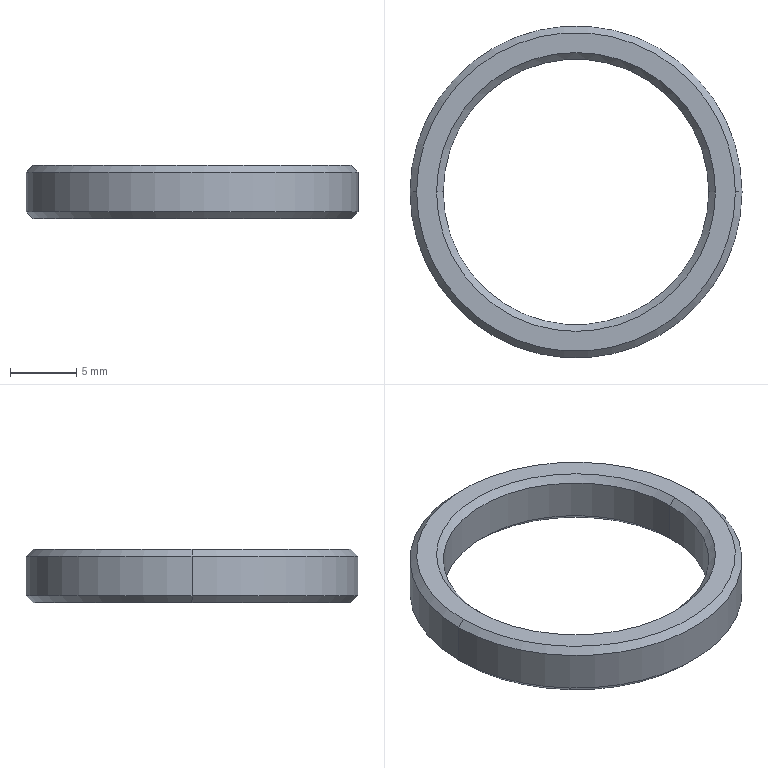Part | SolidWorks | features BaseBody 1 | 1 solid | 14 faces | box 25 x 25 x 4 mm | volume 671.515 mm3 | cone 8 | cylinder 4 | plane 2 | commonest cylinder face diameters 20 x2 25 x2
STEP:
#1=CARTESIAN_POINT('',(-10.,0.,1.5));
#2=VERTEX_POINT('',#1);
#3=CARTESIAN_POINT('',(10.,0.,1.5));
#4=VERTEX_POINT('',#3);
#5=CARTESIAN_POINT('',(0.,0.,1.5));
#6=DIRECTION('',(0.,0.,1.));
#7=DIRECTION('',(1.,0.,0.));
#8=AXIS2_PLACEMENT_3D('',#5,#6,#7);
#9=CIRCLE('',#8,10.);
#10=EDGE_CURVE('',#2,#4,#9,.T.);
#11=ORIENTED_EDGE('',*,*,#10,.F.);
#12=CARTESIAN_POINT('',(-10.5,0.,2.));
#13=VERTEX_POINT('',#12);
#14=CARTESIAN_POINT('',(-10.,0.,1.5));
#15=DIRECTION('',(-0.7071,0.,0.7071));
#16=VECTOR('',#15,1000.);
#17=LINE('',#14,#16);
#18=EDGE_CURVE('',#2,#13,#17,.T.);
#19=ORIENTED_EDGE('',*,*,#18,.T.);
#20=CARTESIAN_POINT('',(10.5,0.,2.));
#21=VERTEX_POINT('',#20);
#22=CARTESIAN_POINT('',(0.,0.,2.));
#23=DIRECTION('',(0.,0.,-1.));
#24=DIRECTION('',(1.,0.,0.));
#25=AXIS2_PLACEMENT_3D('',#22,#23,#24);
#26=CIRCLE('',#25,10.5);
#27=EDGE_CURVE('',#21,#13,#26,.T.);
#28=ORIENTED_EDGE('',*,*,#27,.F.);
#29=CARTESIAN_POINT('',(10.,0.,1.5));
#30=DIRECTION('',(0.7071,0.,0.7071));
#31=VECTOR('',#30,1000.);
#32=LINE('',#29,#31);
#33=EDGE_CURVE('',#4,#21,#32,.T.);
#34=ORIENTED_EDGE('',*,*,#33,.F.);
#35=EDGE_LOOP('',(#11,#19,#28,#34));
#36=FACE_OUTER_BOUND('',#35,.T.);
#37=CARTESIAN_POINT('',(0.,0.,1.5));
#38=DIRECTION('',(0.,0.,1.));
#39=DIRECTION('',(1.,0.,0.));
#40=AXIS2_PLACEMENT_3D('',#37,#38,#39);
#41=CONICAL_SURFACE('',#40,10.,0.7854);
#42=ADVANCED_FACE('',(#36),#41,.F.);
#43=CARTESIAN_POINT('',(10.,0.,-1.5));
#44=VERTEX_POINT('',#43);
#45=CARTESIAN_POINT('',(-10.,0.,-1.5));
#46=VERTEX_POINT('',#45);
#47=CARTESIAN_POINT('',(0.,0.,-1.5));
#48=DIRECTION('',(0.,0.,-1.));
#49=DIRECTION('',(1.,0.,0.));
#50=AXIS2_PLACEMENT_3D('',#47,#48,#49);
#51=CIRCLE('',#50,10.);
#52=EDGE_CURVE('',#44,#46,#51,.T.);
#53=ORIENTED_EDGE('',*,*,#52,.F.);
#54=CARTESIAN_POINT('',(10.5,0.,-2.));
#55=VERTEX_POINT('',#54);
#56=CARTESIAN_POINT('',(10.5,0.,-2.));
#57=DIRECTION('',(0.7071,0.,-0.7071));
#58=VECTOR('',#57,1000.);
#59=LINE('',#56,#58);
#60=EDGE_CURVE('',#44,#55,#59,.T.);
#61=ORIENTED_EDGE('',*,*,#60,.T.);
#62=CARTESIAN_POINT('',(-10.5,0.,-2.));
#63=VERTEX_POINT('',#62);
#64=CARTESIAN_POINT('',(0.,0.,-2.));
#65=DIRECTION('',(0.,0.,1.));
#66=DIRECTION('',(1.,0.,0.));
#67=AXIS2_PLACEMENT_3D('',#64,#65,#66);
#68=CIRCLE('',#67,10.5);
#69=EDGE_CURVE('',#63,#55,#68,.T.);
#70=ORIENTED_EDGE('',*,*,#69,.F.);
#71=CARTESIAN_POINT('',(-10.5,0.,-2.));
#72=DIRECTION('',(-0.7071,0.,-0.7071));
#73=VECTOR('',#72,1000.);
#74=LINE('',#71,#73);
#75=EDGE_CURVE('',#46,#63,#74,.T.);
#76=ORIENTED_EDGE('',*,*,#75,.F.);
#77=EDGE_LOOP('',(#53,#61,#70,#76));
#78=FACE_OUTER_BOUND('',#77,.T.);
#79=CARTESIAN_POINT('',(0.,0.,-2.));
#80=DIRECTION('',(0.,0.,-1.));
#81=DIRECTION('',(-1.,0.,0.));
#82=AXIS2_PLACEMENT_3D('',#79,#80,#81);
#83=CONICAL_SURFACE('',#82,10.5,0.7854);
#84=ADVANCED_FACE('',(#78),#83,.F.);
#85=CARTESIAN_POINT('',(12.,0.,2.));
#86=VERTEX_POINT('',#85);
#87=CARTESIAN_POINT('',(-12.,0.,2.));
#88=VERTEX_POINT('',#87);
#89=CARTESIAN_POINT('',(0.,0.,2.));
#90=DIRECTION('',(0.,0.,1.));
#91=DIRECTION('',(1.,0.,0.));
#92=AXIS2_PLACEMENT_3D('',#89,#90,#91);
#93=CIRCLE('',#92,12.);
#94=EDGE_CURVE('',#86,#88,#93,.T.);
#95=ORIENTED_EDGE('',*,*,#94,.F.);
#96=CARTESIAN_POINT('',(12.5,0.,1.5));
#97=VERTEX_POINT('',#96);
#98=CARTESIAN_POINT('',(12.,0.,2.));
#99=DIRECTION('',(0.7071,0.,-0.7071));
#100=VECTOR('',#99,1000.);
#101=LINE('',#98,#100);
#102=EDGE_CURVE('',#86,#97,#101,.T.);
#103=ORIENTED_EDGE('',*,*,#102,.T.);
#104=CARTESIAN_POINT('',(-12.5,0.,1.5));
#105=VERTEX_POINT('',#104);
#106=CARTESIAN_POINT('',(0.,0.,1.5));
#107=DIRECTION('',(0.,0.,-1.));
#108=DIRECTION('',(1.,0.,0.));
#109=AXIS2_PLACEMENT_3D('',#106,#107,#108);
#110=CIRCLE('',#109,12.5);
#111=EDGE_CURVE('',#105,#97,#110,.T.);
#112=ORIENTED_EDGE('',*,*,#111,.F.);
#113=CARTESIAN_POINT('',(-12.,0.,2.));
#114=DIRECTION('',(-0.7071,0.,-0.7071));
#115=VECTOR('',#114,1000.);
#116=LINE('',#113,#115);
#117=EDGE_CURVE('',#88,#105,#116,.T.);
#118=ORIENTED_EDGE('',*,*,#117,.F.);
#119=EDGE_LOOP('',(#95,#103,#112,#118));
#120=FACE_OUTER_BOUND('',#119,.T.);
#121=CARTESIAN_POINT('',(0.,0.,2.));
#122=DIRECTION('',(0.,0.,-1.));
#123=DIRECTION('',(-1.,0.,0.));
#124=AXIS2_PLACEMENT_3D('',#121,#122,#123);
#125=CONICAL_SURFACE('',#124,12.,0.7854);
#126=ADVANCED_FACE('',(#120),#125,.T.);
#127=CARTESIAN_POINT('',(-12.,0.,-2.));
#128=VERTEX_POINT('',#127);
#129=CARTESIAN_POINT('',(12.,0.,-2.));
#130=VERTEX_POINT('',#129);
#131=CARTESIAN_POINT('',(0.,0.,-2.));
#132=DIRECTION('',(0.,0.,-1.));
#133=DIRECTION('',(1.,0.,0.));
#134=AXIS2_PLACEMENT_3D('',#131,#132,#133);
#135=CIRCLE('',#134,12.);
#136=EDGE_CURVE('',#128,#130,#135,.T.);
#137=ORIENTED_EDGE('',*,*,#136,.F.);
#138=CARTESIAN_POINT('',(-12.5,0.,-1.5));
#139=VERTEX_POINT('',#138);
#140=CARTESIAN_POINT('',(-12.5,0.,-1.5));
#141=DIRECTION('',(-0.7071,0.,0.7071));
#142=VECTOR('',#141,1000.);
#143=LINE('',#140,#142);
#144=EDGE_CURVE('',#128,#139,#143,.T.);
#145=ORIENTED_EDGE('',*,*,#144,.T.);
#146=CARTESIAN_POINT('',(12.5,0.,-1.5));
#147=VERTEX_POINT('',#146);
#148=CARTESIAN_POINT('',(0.,0.,-1.5));
#149=DIRECTION('',(0.,0.,1.));
#150=DIRECTION('',(1.,0.,0.));
#151=AXIS2_PLACEMENT_3D('',#148,#149,#150);
#152=CIRCLE('',#151,12.5);
#153=EDGE_CURVE('',#147,#139,#152,.T.);
#154=ORIENTED_EDGE('',*,*,#153,.F.);
#155=CARTESIAN_POINT('',(12.5,0.,-1.5));
#156=DIRECTION('',(0.7071,0.,0.7071));
#157=VECTOR('',#156,1000.);
#158=LINE('',#155,#157);
#159=EDGE_CURVE('',#130,#147,#158,.T.);
#160=ORIENTED_EDGE('',*,*,#159,.F.);
#161=EDGE_LOOP('',(#137,#145,#154,#160));
#162=FACE_OUTER_BOUND('',#161,.T.);
#163=CARTESIAN_POINT('',(0.,0.,-1.5));
#164=DIRECTION('',(0.,0.,1.));
#165=DIRECTION('',(1.,0.,0.));
#166=AXIS2_PLACEMENT_3D('',#163,#164,#165);
#167=CONICAL_SURFACE('',#166,12.5,0.7854);
#168=ADVANCED_FACE('',(#162),#167,.T.);
#169=ORIENTED_EDGE('',*,*,#10,.T.);
#170=CARTESIAN_POINT('',(10.,0.,2.));
#171=DIRECTION('',(0.,0.,-1.));
#172=VECTOR('',#171,1000.);
#173=LINE('',#170,#172);
#174=EDGE_CURVE('',#4,#44,#173,.T.);
#175=ORIENTED_EDGE('',*,*,#174,.T.);
#176=ORIENTED_EDGE('',*,*,#52,.T.);
#177=CARTESIAN_POINT('',(-10.,0.,2.));
#178=DIRECTION('',(0.,0.,-1.));
#179=VECTOR('',#178,1000.);
#180=LINE('',#177,#179);
#181=EDGE_CURVE('',#2,#46,#180,.T.);
#182=ORIENTED_EDGE('',*,*,#181,.F.);
#183=EDGE_LOOP('',(#169,#175,#176,#182));
#184=FACE_OUTER_BOUND('',#183,.T.);
#185=CARTESIAN_POINT('',(0.,0.,2.));
#186=DIRECTION('',(0.,0.,-1.));
#187=DIRECTION('',(-1.,0.,0.));
#188=AXIS2_PLACEMENT_3D('',#185,#186,#187);
#189=CYLINDRICAL_SURFACE('',#188,10.);
#190=ADVANCED_FACE('',(#184),#189,.F.);
#191=ORIENTED_EDGE('',*,*,#111,.T.);
#192=CARTESIAN_POINT('',(12.5,0.,2.));
#193=DIRECTION('',(0.,0.,-1.));
#194=VECTOR('',#193,1000.);
#195=LINE('',#192,#194);
#196=EDGE_CURVE('',#97,#147,#195,.T.);
#197=ORIENTED_EDGE('',*,*,#196,.T.);
#198=ORIENTED_EDGE('',*,*,#153,.T.);
#199=CARTESIAN_POINT('',(-12.5,0.,2.));
#200=DIRECTION('',(0.,0.,-1.));
#201=VECTOR('',#200,1000.);
#202=LINE('',#199,#201);
#203=EDGE_CURVE('',#105,#139,#202,.T.);
#204=ORIENTED_EDGE('',*,*,#203,.F.);
#205=EDGE_LOOP('',(#191,#197,#198,#204));
#206=FACE_OUTER_BOUND('',#205,.T.);
#207=CARTESIAN_POINT('',(0.,0.,2.));
#208=DIRECTION('',(0.,0.,-1.));
#209=DIRECTION('',(-1.,0.,0.));
#210=AXIS2_PLACEMENT_3D('',#207,#208,#209);
#211=CYLINDRICAL_SURFACE('',#210,12.5);
#212=ADVANCED_FACE('',(#206),#211,.T.);
#213=ORIENTED_EDGE('',*,*,#69,.T.);
#214=CARTESIAN_POINT('',(0.,0.,-2.));
#215=DIRECTION('',(0.,0.,1.));
#216=DIRECTION('',(1.,0.,0.));
#217=AXIS2_PLACEMENT_3D('',#214,#215,#216);
#218=CIRCLE('',#217,10.5);
#219=EDGE_CURVE('',#55,#63,#218,.T.);
#220=ORIENTED_EDGE('',*,*,#219,.T.);
#221=EDGE_LOOP('',(#213,#220));
#222=FACE_BOUND('',#221,.T.);
#223=CARTESIAN_POINT('',(0.,0.,-2.));
#224=DIRECTION('',(0.,0.,-1.));
#225=DIRECTION('',(1.,0.,0.));
#226=AXIS2_PLACEMENT_3D('',#223,#224,#225);
#227=CIRCLE('',#226,12.);
#228=EDGE_CURVE('',#130,#128,#227,.T.);
#229=ORIENTED_EDGE('',*,*,#228,.T.);
#230=ORIENTED_EDGE('',*,*,#136,.T.);
#231=EDGE_LOOP('',(#229,#230));
#232=FACE_OUTER_BOUND('',#231,.T.);
#233=CARTESIAN_POINT('',(0.,0.,-2.));
#234=DIRECTION('',(0.,0.,1.));
#235=DIRECTION('',(1.,0.,0.));
#236=AXIS2_PLACEMENT_3D('',#233,#234,#235);
#237=PLANE('',#236);
#238=ADVANCED_FACE('',(#222,#232),#237,.F.);
#239=ORIENTED_EDGE('',*,*,#27,.T.);
#240=CARTESIAN_POINT('',(0.,0.,2.));
#241=DIRECTION('',(0.,0.,-1.));
#242=DIRECTION('',(1.,0.,0.));
#243=AXIS2_PLACEMENT_3D('',#240,#241,#242);
#244=CIRCLE('',#243,10.5);
#245=EDGE_CURVE('',#13,#21,#244,.T.);
#246=ORIENTED_EDGE('',*,*,#245,.T.);
#247=EDGE_LOOP('',(#239,#246));
#248=FACE_BOUND('',#247,.T.);
#249=CARTESIAN_POINT('',(0.,0.,2.));
#250=DIRECTION('',(0.,0.,1.));
#251=DIRECTION('',(1.,0.,0.));
#252=AXIS2_PLACEMENT_3D('',#249,#250,#251);
#253=CIRCLE('',#252,12.);
#254=EDGE_CURVE('',#88,#86,#253,.T.);
#255=ORIENTED_EDGE('',*,*,#254,.T.);
#256=ORIENTED_EDGE('',*,*,#94,.T.);
#257=EDGE_LOOP('',(#255,#256));
#258=FACE_OUTER_BOUND('',#257,.T.);
#259=CARTESIAN_POINT('',(0.,0.,2.));
#260=DIRECTION('',(0.,0.,1.));
#261=DIRECTION('',(1.,0.,0.));
#262=AXIS2_PLACEMENT_3D('',#259,#260,#261);
#263=PLANE('',#262);
#264=ADVANCED_FACE('',(#248,#258),#263,.T.);
#265=ORIENTED_EDGE('',*,*,#196,.F.);
#266=CARTESIAN_POINT('',(0.,0.,1.5));
#267=DIRECTION('',(0.,0.,-1.));
#268=DIRECTION('',(1.,0.,0.));
#269=AXIS2_PLACEMENT_3D('',#266,#267,#268);
#270=CIRCLE('',#269,12.5);
#271=EDGE_CURVE('',#97,#105,#270,.T.);
#272=ORIENTED_EDGE('',*,*,#271,.T.);
#273=ORIENTED_EDGE('',*,*,#203,.T.);
#274=CARTESIAN_POINT('',(0.,0.,-1.5));
#275=DIRECTION('',(0.,0.,1.));
#276=DIRECTION('',(1.,0.,0.));
#277=AXIS2_PLACEMENT_3D('',#274,#275,#276);
#278=CIRCLE('',#277,12.5);
#279=EDGE_CURVE('',#139,#147,#278,.T.);
#280=ORIENTED_EDGE('',*,*,#279,.T.);
#281=EDGE_LOOP('',(#265,#272,#273,#280));
#282=FACE_OUTER_BOUND('',#281,.T.);
#283=CARTESIAN_POINT('',(0.,0.,2.));
#284=DIRECTION('',(0.,0.,-1.));
#285=DIRECTION('',(-1.,0.,0.));
#286=AXIS2_PLACEMENT_3D('',#283,#284,#285);
#287=CYLINDRICAL_SURFACE('',#286,12.5);
#288=ADVANCED_FACE('',(#282),#287,.T.);
#289=ORIENTED_EDGE('',*,*,#174,.F.);
#290=CARTESIAN_POINT('',(0.,0.,1.5));
#291=DIRECTION('',(0.,0.,1.));
#292=DIRECTION('',(1.,0.,0.));
#293=AXIS2_PLACEMENT_3D('',#290,#291,#292);
#294=CIRCLE('',#293,10.);
#295=EDGE_CURVE('',#4,#2,#294,.T.);
#296=ORIENTED_EDGE('',*,*,#295,.T.);
#297=ORIENTED_EDGE('',*,*,#181,.T.);
#298=CARTESIAN_POINT('',(0.,0.,-1.5));
#299=DIRECTION('',(0.,0.,-1.));
#300=DIRECTION('',(1.,0.,0.));
#301=AXIS2_PLACEMENT_3D('',#298,#299,#300);
#302=CIRCLE('',#301,10.);
#303=EDGE_CURVE('',#46,#44,#302,.T.);
#304=ORIENTED_EDGE('',*,*,#303,.T.);
#305=EDGE_LOOP('',(#289,#296,#297,#304));
#306=FACE_OUTER_BOUND('',#305,.T.);
#307=CARTESIAN_POINT('',(0.,0.,2.));
#308=DIRECTION('',(0.,0.,-1.));
#309=DIRECTION('',(-1.,0.,0.));
#310=AXIS2_PLACEMENT_3D('',#307,#308,#309);
#311=CYLINDRICAL_SURFACE('',#310,10.);
#312=ADVANCED_FACE('',(#306),#311,.F.);
#313=ORIENTED_EDGE('',*,*,#144,.F.);
#314=ORIENTED_EDGE('',*,*,#228,.F.);
#315=ORIENTED_EDGE('',*,*,#159,.T.);
#316=ORIENTED_EDGE('',*,*,#279,.F.);
#317=EDGE_LOOP('',(#313,#314,#315,#316));
#318=FACE_OUTER_BOUND('',#317,.T.);
#319=CARTESIAN_POINT('',(0.,0.,-1.5));
#320=DIRECTION('',(0.,0.,1.));
#321=DIRECTION('',(1.,0.,0.));
#322=AXIS2_PLACEMENT_3D('',#319,#320,#321);
#323=CONICAL_SURFACE('',#322,12.5,0.7854);
#324=ADVANCED_FACE('',(#318),#323,.T.);
#325=ORIENTED_EDGE('',*,*,#102,.F.);
#326=ORIENTED_EDGE('',*,*,#254,.F.);
#327=ORIENTED_EDGE('',*,*,#117,.T.);
#328=ORIENTED_EDGE('',*,*,#271,.F.);
#329=EDGE_LOOP('',(#325,#326,#327,#328));
#330=FACE_OUTER_BOUND('',#329,.T.);
#331=CARTESIAN_POINT('',(0.,0.,2.));
#332=DIRECTION('',(0.,0.,-1.));
#333=DIRECTION('',(-1.,0.,0.));
#334=AXIS2_PLACEMENT_3D('',#331,#332,#333);
#335=CONICAL_SURFACE('',#334,12.,0.7854);
#336=ADVANCED_FACE('',(#330),#335,.T.);
#337=ORIENTED_EDGE('',*,*,#60,.F.);
#338=ORIENTED_EDGE('',*,*,#303,.F.);
#339=ORIENTED_EDGE('',*,*,#75,.T.);
#340=ORIENTED_EDGE('',*,*,#219,.F.);
#341=EDGE_LOOP('',(#337,#338,#339,#340));
#342=FACE_OUTER_BOUND('',#341,.T.);
#343=CARTESIAN_POINT('',(0.,0.,-2.));
#344=DIRECTION('',(0.,0.,-1.));
#345=DIRECTION('',(-1.,0.,0.));
#346=AXIS2_PLACEMENT_3D('',#343,#344,#345);
#347=CONICAL_SURFACE('',#346,10.5,0.7854);
#348=ADVANCED_FACE('',(#342),#347,.F.);
#349=ORIENTED_EDGE('',*,*,#18,.F.);
#350=ORIENTED_EDGE('',*,*,#295,.F.);
#351=ORIENTED_EDGE('',*,*,#33,.T.);
#352=ORIENTED_EDGE('',*,*,#245,.F.);
#353=EDGE_LOOP('',(#349,#350,#351,#352));
#354=FACE_OUTER_BOUND('',#353,.T.);
#355=CARTESIAN_POINT('',(0.,0.,1.5));
#356=DIRECTION('',(0.,0.,1.));
#357=DIRECTION('',(1.,0.,0.));
#358=AXIS2_PLACEMENT_3D('',#355,#356,#357);
#359=CONICAL_SURFACE('',#358,10.,0.7854);
#360=ADVANCED_FACE('',(#354),#359,.F.);
#361=CLOSED_SHELL('',(#42,#84,#126,#168,#190,#212,#238,#264,#288,#312,#324,#336,#348,#360));
#362=MANIFOLD_SOLID_BREP('',#361);
#363=CARTESIAN_POINT('',(0.,0.,0.));
#364=DIRECTION('',(0.,0.,1.));
#365=DIRECTION('',(1.,0.,0.));
#366=AXIS2_PLACEMENT_3D('',#363,#364,#365);
#367=(LENGTH_UNIT()NAMED_UNIT(*)SI_UNIT(.MILLI.,.METRE.));
#368=UNCERTAINTY_MEASURE_WITH_UNIT(LENGTH_MEASURE(0.00001),#367,'','');
#369=(NAMED_UNIT(*)PLANE_ANGLE_UNIT()SI_UNIT($,.RADIAN.));
#370=(NAMED_UNIT(*)SI_UNIT($,.STERADIAN.)SOLID_ANGLE_UNIT());
#371=(GEOMETRIC_REPRESENTATION_CONTEXT(3)GLOBAL_UNCERTAINTY_ASSIGNED_CONTEXT((#368))GLOBAL_UNIT_ASSIGNED_CONTEXT((#367,#369,#370))REPRESENTATION_CONTEXT('',''));
#372=ADVANCED_BREP_SHAPE_REPRESENTATION('',(#362,#366),#371);